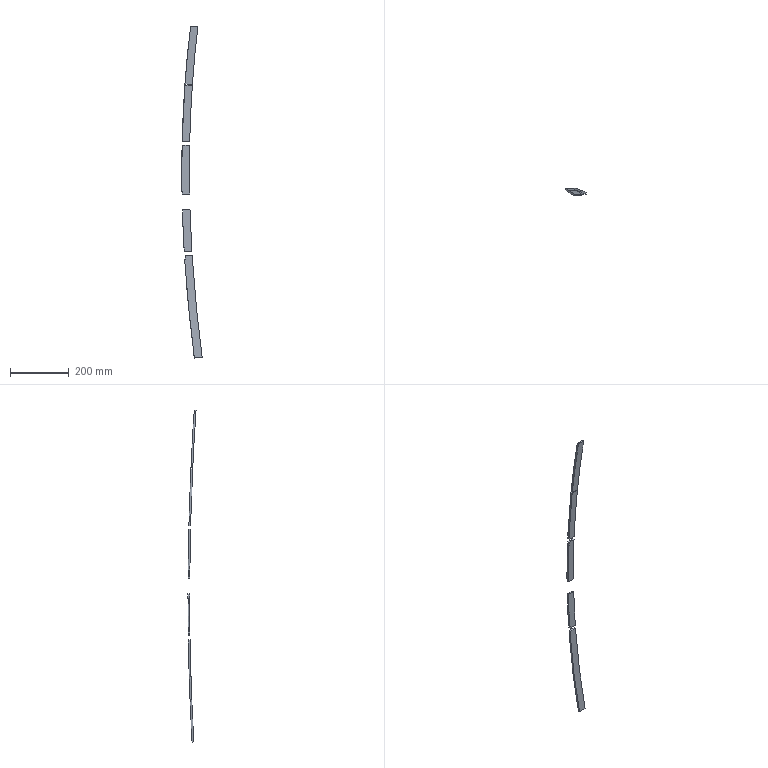Part | SolidWorks | features BaseBody 5 | 5 solids | 42 faces | box 69.314 x 27.238 x 1130 mm | volume 155558 mm3 | plane 22 | spline 20